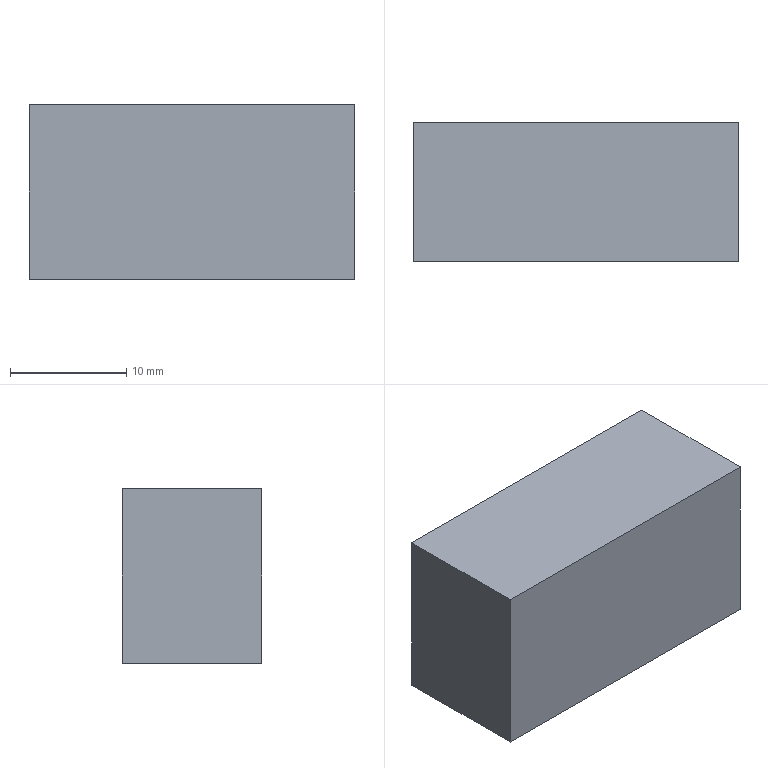Part | NX | features solid 2 | 1 solid | 6 faces | box 28 x 12 x 15 mm | volume 5040 mm3 | plane 6
STEP:
#1=CARTESIAN_POINT('',(-887.,-238.5,-35.));
#2=VERTEX_POINT('',#1);
#3=CARTESIAN_POINT('',(-915.,-238.5,-35.));
#4=VERTEX_POINT('',#3);
#5=CARTESIAN_POINT('',(-979.,-238.5,-35.));
#6=DIRECTION('',(-1.,0.,0.));
#7=VECTOR('',#6,1000.);
#8=LINE('',#5,#7);
#9=EDGE_CURVE('',#2,#4,#8,.T.);
#10=ORIENTED_EDGE('',*,*,#9,.F.);
#11=CARTESIAN_POINT('',(-887.,-238.5,-20.));
#12=VERTEX_POINT('',#11);
#13=CARTESIAN_POINT('',(-887.,-238.5,54.523));
#14=DIRECTION('',(0.,0.,1.));
#15=VECTOR('',#14,1000.);
#16=LINE('',#13,#15);
#17=EDGE_CURVE('',#2,#12,#16,.T.);
#18=ORIENTED_EDGE('',*,*,#17,.T.);
#19=CARTESIAN_POINT('',(-915.,-238.5,-20.));
#20=VERTEX_POINT('',#19);
#21=CARTESIAN_POINT('',(-979.,-238.5,-20.));
#22=DIRECTION('',(1.,0.,0.));
#23=VECTOR('',#22,1000.);
#24=LINE('',#21,#23);
#25=EDGE_CURVE('',#20,#12,#24,.T.);
#26=ORIENTED_EDGE('',*,*,#25,.F.);
#27=CARTESIAN_POINT('',(-915.,-238.5,-10.));
#28=DIRECTION('',(0.,0.,-1.));
#29=VECTOR('',#28,1000.);
#30=LINE('',#27,#29);
#31=EDGE_CURVE('',#20,#4,#30,.T.);
#32=ORIENTED_EDGE('',*,*,#31,.T.);
#33=EDGE_LOOP('',(#10,#18,#26,#32));
#34=FACE_BOUND('',#33,.T.);
#35=CARTESIAN_POINT('',(-979.,-238.5,54.523));
#36=DIRECTION('',(0.,1.,0.));
#37=DIRECTION('',(1.,0.,0.));
#38=AXIS2_PLACEMENT_3D('',#35,#36,#37);
#39=PLANE('',#38);
#40=ADVANCED_FACE('',(#34),#39,.F.);
#41=CARTESIAN_POINT('',(-887.,-226.5,-35.));
#42=VERTEX_POINT('',#41);
#43=CARTESIAN_POINT('',(-887.,-226.5,-20.));
#44=VERTEX_POINT('',#43);
#45=CARTESIAN_POINT('',(-887.,-226.5,54.523));
#46=DIRECTION('',(0.,0.,1.));
#47=VECTOR('',#46,1000.);
#48=LINE('',#45,#47);
#49=EDGE_CURVE('',#42,#44,#48,.T.);
#50=ORIENTED_EDGE('',*,*,#49,.F.);
#51=CARTESIAN_POINT('',(-915.,-226.5,-35.));
#52=VERTEX_POINT('',#51);
#53=CARTESIAN_POINT('',(-979.,-226.5,-35.));
#54=DIRECTION('',(-1.,0.,0.));
#55=VECTOR('',#54,1000.);
#56=LINE('',#53,#55);
#57=EDGE_CURVE('',#42,#52,#56,.T.);
#58=ORIENTED_EDGE('',*,*,#57,.T.);
#59=CARTESIAN_POINT('',(-915.,-226.5,-20.));
#60=VERTEX_POINT('',#59);
#61=CARTESIAN_POINT('',(-915.,-226.5,-35.));
#62=DIRECTION('',(0.,0.,1.));
#63=VECTOR('',#62,1000.);
#64=LINE('',#61,#63);
#65=EDGE_CURVE('',#52,#60,#64,.T.);
#66=ORIENTED_EDGE('',*,*,#65,.T.);
#67=CARTESIAN_POINT('',(-1002.,-226.5,-20.));
#68=DIRECTION('',(-1.,0.,0.));
#69=VECTOR('',#68,1000.);
#70=LINE('',#67,#69);
#71=EDGE_CURVE('',#44,#60,#70,.T.);
#72=ORIENTED_EDGE('',*,*,#71,.F.);
#73=EDGE_LOOP('',(#50,#58,#66,#72));
#74=FACE_BOUND('',#73,.T.);
#75=CARTESIAN_POINT('',(-979.,-226.5,54.523));
#76=DIRECTION('',(0.,1.,0.));
#77=DIRECTION('',(1.,0.,0.));
#78=AXIS2_PLACEMENT_3D('',#75,#76,#77);
#79=PLANE('',#78);
#80=ADVANCED_FACE('',(#74),#79,.T.);
#81=ORIENTED_EDGE('',*,*,#71,.T.);
#82=CARTESIAN_POINT('',(-915.,-226.5,-20.));
#83=DIRECTION('',(0.,1.,0.));
#84=VECTOR('',#83,1000.);
#85=LINE('',#82,#84);
#86=EDGE_CURVE('',#20,#60,#85,.T.);
#87=ORIENTED_EDGE('',*,*,#86,.F.);
#88=ORIENTED_EDGE('',*,*,#25,.T.);
#89=CARTESIAN_POINT('',(-887.,-77.5,-20.));
#90=DIRECTION('',(0.,1.,0.));
#91=VECTOR('',#90,1000.);
#92=LINE('',#89,#91);
#93=EDGE_CURVE('',#12,#44,#92,.T.);
#94=ORIENTED_EDGE('',*,*,#93,.T.);
#95=EDGE_LOOP('',(#81,#87,#88,#94));
#96=FACE_BOUND('',#95,.T.);
#97=CARTESIAN_POINT('',(-932.,-124.5,-20.));
#98=DIRECTION('',(0.,0.,1.));
#99=DIRECTION('',(1.,0.,0.));
#100=AXIS2_PLACEMENT_3D('',#97,#98,#99);
#101=PLANE('',#100);
#102=ADVANCED_FACE('',(#96),#101,.T.);
#103=CARTESIAN_POINT('',(-915.,-226.5,-35.));
#104=DIRECTION('',(0.,1.,0.));
#105=VECTOR('',#104,1000.);
#106=LINE('',#103,#105);
#107=EDGE_CURVE('',#4,#52,#106,.T.);
#108=ORIENTED_EDGE('',*,*,#107,.T.);
#109=ORIENTED_EDGE('',*,*,#57,.F.);
#110=CARTESIAN_POINT('',(-887.,-124.5,-35.));
#111=DIRECTION('',(0.,-1.,0.));
#112=VECTOR('',#111,1000.);
#113=LINE('',#110,#112);
#114=EDGE_CURVE('',#42,#2,#113,.T.);
#115=ORIENTED_EDGE('',*,*,#114,.T.);
#116=ORIENTED_EDGE('',*,*,#9,.T.);
#117=EDGE_LOOP('',(#108,#109,#115,#116));
#118=FACE_BOUND('',#117,.T.);
#119=CARTESIAN_POINT('',(-932.,-124.5,-35.));
#120=DIRECTION('',(0.,0.,1.));
#121=DIRECTION('',(1.,0.,0.));
#122=AXIS2_PLACEMENT_3D('',#119,#120,#121);
#123=PLANE('',#122);
#124=ADVANCED_FACE('',(#118),#123,.F.);
#125=ORIENTED_EDGE('',*,*,#65,.F.);
#126=ORIENTED_EDGE('',*,*,#107,.F.);
#127=ORIENTED_EDGE('',*,*,#31,.F.);
#128=ORIENTED_EDGE('',*,*,#86,.T.);
#129=EDGE_LOOP('',(#125,#126,#127,#128));
#130=FACE_BOUND('',#129,.T.);
#131=CARTESIAN_POINT('',(-915.,-226.5,-35.));
#132=DIRECTION('',(-1.,0.,0.));
#133=DIRECTION('',(0.,0.,1.));
#134=AXIS2_PLACEMENT_3D('',#131,#132,#133);
#135=PLANE('',#134);
#136=ADVANCED_FACE('',(#130),#135,.T.);
#137=ORIENTED_EDGE('',*,*,#17,.F.);
#138=ORIENTED_EDGE('',*,*,#114,.F.);
#139=ORIENTED_EDGE('',*,*,#49,.T.);
#140=ORIENTED_EDGE('',*,*,#93,.F.);
#141=EDGE_LOOP('',(#137,#138,#139,#140));
#142=FACE_BOUND('',#141,.T.);
#143=CARTESIAN_POINT('',(-887.,-238.5,-20.));
#144=DIRECTION('',(-1.,0.,0.));
#145=DIRECTION('',(0.,-1.,0.));
#146=AXIS2_PLACEMENT_3D('',#143,#144,#145);
#147=PLANE('',#146);
#148=ADVANCED_FACE('',(#142),#147,.F.);
#149=CLOSED_SHELL('',(#40,#80,#102,#124,#136,#148));
#150=MANIFOLD_SOLID_BREP('',#149);
#151=(LENGTH_UNIT()NAMED_UNIT(*)SI_UNIT(.MILLI.,.METRE.));
#152=UNCERTAINTY_MEASURE_WITH_UNIT(LENGTH_MEASURE(0.00001),#151,'','');
#153=(NAMED_UNIT(*)PLANE_ANGLE_UNIT()SI_UNIT($,.RADIAN.));
#154=(NAMED_UNIT(*)SI_UNIT($,.STERADIAN.)SOLID_ANGLE_UNIT());
#155=(GEOMETRIC_REPRESENTATION_CONTEXT(3)GLOBAL_UNCERTAINTY_ASSIGNED_CONTEXT((#152))GLOBAL_UNIT_ASSIGNED_CONTEXT((#151,#153,#154))REPRESENTATION_CONTEXT('',''));
#156=ADVANCED_BREP_SHAPE_REPRESENTATION('',(#150),#155);